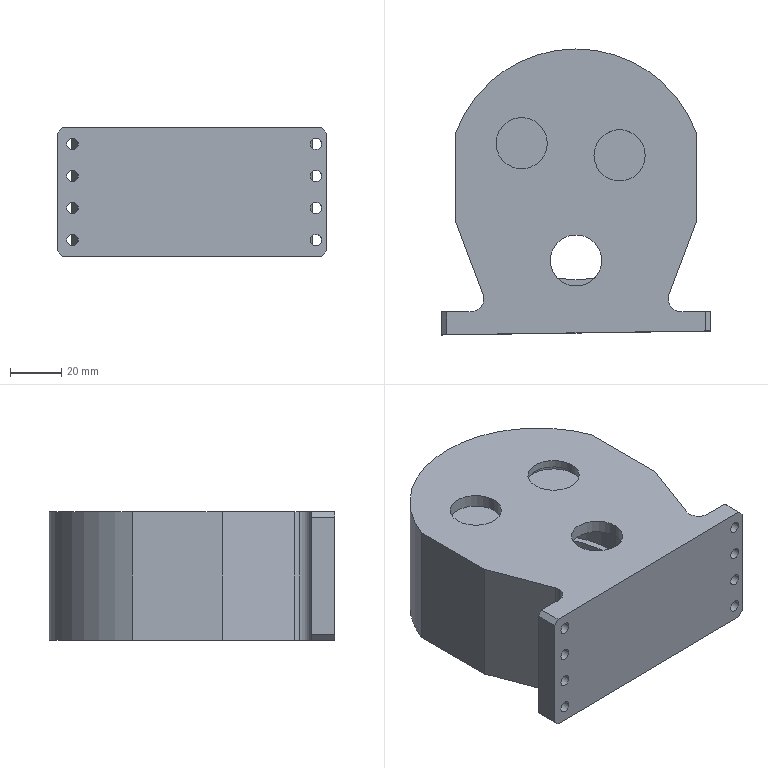Part | SolidWorks | features ICE 10, Fillet 2, Chamfer 1, Extrusion 1 | 1 solid | 84 faces | box 105 x 111.51 x 50 mm | volume 200027 mm3 | cylinder 55 | plane 29 | commonest cylinder face diameters 4 x20 4.5 x16 20 x6 10 x3 8 x2 25 x2